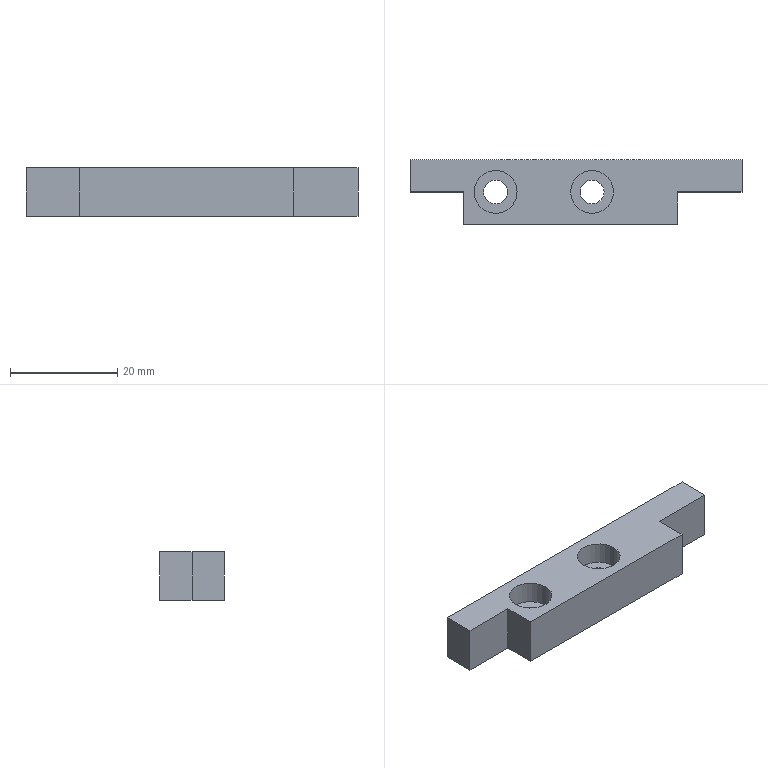Part | STEP file | BU-B02 | 1 solid | 20 faces | box 62 x 12 x 9 mm | volume 4933 mm3 | plane 12 | cylinder 8 | commonest cylinder face diameters 4.5 x4 8 x4
STEP:
#1=CARTESIAN_POINT('',(0.,0.,0.));
#2=DIRECTION('',(0.,0.,1.));
#3=DIRECTION('',(1.,0.,0.));
#4=AXIS2_PLACEMENT_3D('',#1,#2,#3);
#5=CARTESIAN_POINT('',(80.562,56.025,4.8));
#6=VERTEX_POINT('',#5);
#7=CARTESIAN_POINT('',(80.562,56.025,9.));
#8=VERTEX_POINT('',#7);
#9=CARTESIAN_POINT('',(80.562,56.025,9.));
#10=DIRECTION('',(0.,0.,1.));
#11=VECTOR('',#10,1.);
#12=LINE('',#9,#11);
#13=CARTESIAN_POINT('',(76.562,56.025,9.));
#14=DIRECTION('',(0.,0.,1.));
#15=DIRECTION('',(1.,0.,0.));
#16=AXIS2_PLACEMENT_3D('',#13,#14,#15);
#17=CYLINDRICAL_SURFACE('',#16,4.);
#18=CARTESIAN_POINT('',(6.283,0.));
#19=DIRECTION('',(0.,1.));
#20=VECTOR('',#19,1.);
#21=LINE('',#18,#20);
#22=(GEOMETRIC_REPRESENTATION_CONTEXT(2)PARAMETRIC_REPRESENTATION_CONTEXT()REPRESENTATION_CONTEXT('',''));
#23=DEFINITIONAL_REPRESENTATION('',(#21),#22);
#24=PCURVE('',#17,#23);
#25=CARTESIAN_POINT('',(76.562,56.025,9.));
#26=DIRECTION('',(0.,0.,1.));
#27=DIRECTION('',(1.,0.,0.));
#28=AXIS2_PLACEMENT_3D('',#25,#26,#27);
#29=CYLINDRICAL_SURFACE('',#28,4.);
#30=CARTESIAN_POINT('',(0.,0.));
#31=DIRECTION('',(0.,1.));
#32=VECTOR('',#31,1.);
#33=LINE('',#30,#32);
#34=(GEOMETRIC_REPRESENTATION_CONTEXT(2)PARAMETRIC_REPRESENTATION_CONTEXT()REPRESENTATION_CONTEXT('',''));
#35=DEFINITIONAL_REPRESENTATION('',(#33),#34);
#36=PCURVE('',#29,#35);
#37=SURFACE_CURVE('',#12,(#24,#36),.PCURVE_S1.);
#38=EDGE_CURVE('',#6,#8,#37,.T.);
#39=ORIENTED_EDGE('',*,*,#38,.T.);
#40=CARTESIAN_POINT('',(72.562,56.025,9.));
#41=VERTEX_POINT('',#40);
#42=CARTESIAN_POINT('',(76.562,56.025,9.));
#43=DIRECTION('',(0.,0.,1.));
#44=DIRECTION('',(1.,0.,0.));
#45=AXIS2_PLACEMENT_3D('',#42,#43,#44);
#46=CIRCLE('',#45,4.);
#47=CARTESIAN_POINT('',(0.,0.));
#48=DIRECTION('',(1.,0.));
#49=VECTOR('',#48,1.);
#50=LINE('',#47,#49);
#51=(GEOMETRIC_REPRESENTATION_CONTEXT(2)PARAMETRIC_REPRESENTATION_CONTEXT()REPRESENTATION_CONTEXT('',''));
#52=DEFINITIONAL_REPRESENTATION('',(#50),#51);
#53=PCURVE('',#17,#52);
#54=CARTESIAN_POINT('',(60.562,62.025,9.));
#55=DIRECTION('',(0.,0.,-1.));
#56=DIRECTION('',(-1.,0.,0.));
#57=AXIS2_PLACEMENT_3D('',#54,#55,#56);
#58=PLANE('',#57);
#59=CARTESIAN_POINT('',(-20.,-6.));
#60=CARTESIAN_POINT('',(-20.,0.9282));
#61=CARTESIAN_POINT('',(-14.,-2.536));
#62=CARTESIAN_POINT('',(-8.,-6.));
#63=CARTESIAN_POINT('',(-14.,-9.464));
#64=CARTESIAN_POINT('',(-20.,-12.928));
#65=CARTESIAN_POINT('',(-20.,-6.));
#66=(BOUNDED_CURVE()B_SPLINE_CURVE(2,(#59,#60,#61,#62,#63,#64,#65),.UNSPECIFIED.,.T.,.F.)B_SPLINE_CURVE_WITH_KNOTS((1,2,2,2,2,1),(-2.094,0.,2.094,4.189,6.283,8.378),.UNSPECIFIED.)CURVE()GEOMETRIC_REPRESENTATION_ITEM()RATIONAL_B_SPLINE_CURVE((1.,0.5,1.,0.5,1.,0.5,1.))REPRESENTATION_ITEM(''));
#67=(GEOMETRIC_REPRESENTATION_CONTEXT(2)PARAMETRIC_REPRESENTATION_CONTEXT()REPRESENTATION_CONTEXT('',''));
#68=DEFINITIONAL_REPRESENTATION('',(#66),#67);
#69=PCURVE('',#58,#68);
#70=SURFACE_CURVE('',#46,(#53,#69),.PCURVE_S1.);
#71=EDGE_CURVE('',#41,#8,#70,.T.);
#72=ORIENTED_EDGE('',*,*,#71,.F.);
#73=CARTESIAN_POINT('',(72.562,56.025,4.8));
#74=VERTEX_POINT('',#73);
#75=CARTESIAN_POINT('',(72.562,56.025,9.));
#76=DIRECTION('',(0.,0.,1.));
#77=VECTOR('',#76,1.);
#78=LINE('',#75,#77);
#79=CARTESIAN_POINT('',(3.142,0.));
#80=DIRECTION('',(0.,1.));
#81=VECTOR('',#80,1.);
#82=LINE('',#79,#81);
#83=(GEOMETRIC_REPRESENTATION_CONTEXT(2)PARAMETRIC_REPRESENTATION_CONTEXT()REPRESENTATION_CONTEXT('',''));
#84=DEFINITIONAL_REPRESENTATION('',(#82),#83);
#85=PCURVE('',#17,#84);
#86=CARTESIAN_POINT('',(3.142,0.));
#87=DIRECTION('',(0.,1.));
#88=VECTOR('',#87,1.);
#89=LINE('',#86,#88);
#90=(GEOMETRIC_REPRESENTATION_CONTEXT(2)PARAMETRIC_REPRESENTATION_CONTEXT()REPRESENTATION_CONTEXT('',''));
#91=DEFINITIONAL_REPRESENTATION('',(#89),#90);
#92=PCURVE('',#29,#91);
#93=SURFACE_CURVE('',#78,(#85,#92),.PCURVE_S1.);
#94=EDGE_CURVE('',#74,#41,#93,.T.);
#95=ORIENTED_EDGE('',*,*,#94,.F.);
#96=CARTESIAN_POINT('',(76.562,56.025,4.8));
#97=DIRECTION('',(0.,0.,1.));
#98=DIRECTION('',(1.,0.,0.));
#99=AXIS2_PLACEMENT_3D('',#96,#97,#98);
#100=CIRCLE('',#99,4.);
#101=CARTESIAN_POINT('',(0.,-4.2));
#102=DIRECTION('',(1.,0.));
#103=VECTOR('',#102,1.);
#104=LINE('',#101,#103);
#105=(GEOMETRIC_REPRESENTATION_CONTEXT(2)PARAMETRIC_REPRESENTATION_CONTEXT()REPRESENTATION_CONTEXT('',''));
#106=DEFINITIONAL_REPRESENTATION('',(#104),#105);
#107=PCURVE('',#17,#106);
#108=CARTESIAN_POINT('',(78.812,56.025,4.8));
#109=DIRECTION('',(0.,0.,-1.));
#110=DIRECTION('',(-1.,0.,0.));
#111=AXIS2_PLACEMENT_3D('',#108,#109,#110);
#112=PLANE('',#111);
#113=CARTESIAN_POINT('',(-1.75,0.));
#114=CARTESIAN_POINT('',(-1.75,6.928));
#115=CARTESIAN_POINT('',(4.25,3.464));
#116=CARTESIAN_POINT('',(10.25,0.));
#117=CARTESIAN_POINT('',(4.25,-3.464));
#118=CARTESIAN_POINT('',(-1.75,-6.928));
#119=CARTESIAN_POINT('',(-1.75,0.));
#120=(BOUNDED_CURVE()B_SPLINE_CURVE(2,(#113,#114,#115,#116,#117,#118,#119),.UNSPECIFIED.,.T.,.F.)B_SPLINE_CURVE_WITH_KNOTS((1,2,2,2,2,1),(-2.094,0.,2.094,4.189,6.283,8.378),.UNSPECIFIED.)CURVE()GEOMETRIC_REPRESENTATION_ITEM()RATIONAL_B_SPLINE_CURVE((1.,0.5,1.,0.5,1.,0.5,1.))REPRESENTATION_ITEM(''));
#121=(GEOMETRIC_REPRESENTATION_CONTEXT(2)PARAMETRIC_REPRESENTATION_CONTEXT()REPRESENTATION_CONTEXT('',''));
#122=DEFINITIONAL_REPRESENTATION('',(#120),#121);
#123=PCURVE('',#112,#122);
#124=SURFACE_CURVE('',#100,(#107,#123),.PCURVE_S1.);
#125=EDGE_CURVE('',#74,#6,#124,.T.);
#126=ORIENTED_EDGE('',*,*,#125,.T.);
#127=EDGE_LOOP('',(#39,#72,#95,#126));
#128=FACE_BOUND('',#127,.F.);
#129=ADVANCED_FACE('',(#128),#17,.F.);
#130=CARTESIAN_POINT('',(78.812,56.025,0.));
#131=VERTEX_POINT('',#130);
#132=CARTESIAN_POINT('',(78.812,56.025,4.8));
#133=VERTEX_POINT('',#132);
#134=CARTESIAN_POINT('',(78.812,56.025,9.));
#135=DIRECTION('',(0.,0.,1.));
#136=VECTOR('',#135,1.);
#137=LINE('',#134,#136);
#138=CARTESIAN_POINT('',(76.562,56.025,9.));
#139=DIRECTION('',(0.,0.,1.));
#140=DIRECTION('',(1.,0.,0.));
#141=AXIS2_PLACEMENT_3D('',#138,#139,#140);
#142=CYLINDRICAL_SURFACE('',#141,2.25);
#143=CARTESIAN_POINT('',(6.283,0.));
#144=DIRECTION('',(0.,1.));
#145=VECTOR('',#144,1.);
#146=LINE('',#143,#145);
#147=(GEOMETRIC_REPRESENTATION_CONTEXT(2)PARAMETRIC_REPRESENTATION_CONTEXT()REPRESENTATION_CONTEXT('',''));
#148=DEFINITIONAL_REPRESENTATION('',(#146),#147);
#149=PCURVE('',#142,#148);
#150=CARTESIAN_POINT('',(76.562,56.025,9.));
#151=DIRECTION('',(0.,0.,1.));
#152=DIRECTION('',(1.,0.,0.));
#153=AXIS2_PLACEMENT_3D('',#150,#151,#152);
#154=CYLINDRICAL_SURFACE('',#153,2.25);
#155=CARTESIAN_POINT('',(0.,0.));
#156=DIRECTION('',(0.,1.));
#157=VECTOR('',#156,1.);
#158=LINE('',#155,#157);
#159=(GEOMETRIC_REPRESENTATION_CONTEXT(2)PARAMETRIC_REPRESENTATION_CONTEXT()REPRESENTATION_CONTEXT('',''));
#160=DEFINITIONAL_REPRESENTATION('',(#158),#159);
#161=PCURVE('',#154,#160);
#162=SURFACE_CURVE('',#137,(#149,#161),.PCURVE_S1.);
#163=EDGE_CURVE('',#131,#133,#162,.T.);
#164=ORIENTED_EDGE('',*,*,#163,.T.);
#165=CARTESIAN_POINT('',(74.312,56.025,4.8));
#166=VERTEX_POINT('',#165);
#167=CARTESIAN_POINT('',(76.562,56.025,4.8));
#168=DIRECTION('',(0.,0.,1.));
#169=DIRECTION('',(1.,0.,0.));
#170=AXIS2_PLACEMENT_3D('',#167,#168,#169);
#171=CIRCLE('',#170,2.25);
#172=CARTESIAN_POINT('',(0.,-4.2));
#173=DIRECTION('',(1.,0.));
#174=VECTOR('',#173,1.);
#175=LINE('',#172,#174);
#176=(GEOMETRIC_REPRESENTATION_CONTEXT(2)PARAMETRIC_REPRESENTATION_CONTEXT()REPRESENTATION_CONTEXT('',''));
#177=DEFINITIONAL_REPRESENTATION('',(#175),#176);
#178=PCURVE('',#142,#177);
#179=CARTESIAN_POINT('',(0.,0.));
#180=CARTESIAN_POINT('',(0.,3.897));
#181=CARTESIAN_POINT('',(3.375,1.949));
#182=CARTESIAN_POINT('',(6.75,0.));
#183=CARTESIAN_POINT('',(3.375,-1.949));
#184=CARTESIAN_POINT('',(0.,-3.897));
#185=CARTESIAN_POINT('',(0.,0.));
#186=(BOUNDED_CURVE()B_SPLINE_CURVE(2,(#179,#180,#181,#182,#183,#184,#185),.UNSPECIFIED.,.T.,.F.)B_SPLINE_CURVE_WITH_KNOTS((1,2,2,2,2,1),(-2.094,0.,2.094,4.189,6.283,8.378),.UNSPECIFIED.)CURVE()GEOMETRIC_REPRESENTATION_ITEM()RATIONAL_B_SPLINE_CURVE((1.,0.5,1.,0.5,1.,0.5,1.))REPRESENTATION_ITEM(''));
#187=(GEOMETRIC_REPRESENTATION_CONTEXT(2)PARAMETRIC_REPRESENTATION_CONTEXT()REPRESENTATION_CONTEXT('',''));
#188=DEFINITIONAL_REPRESENTATION('',(#186),#187);
#189=PCURVE('',#112,#188);
#190=SURFACE_CURVE('',#171,(#178,#189),.PCURVE_S1.);
#191=EDGE_CURVE('',#166,#133,#190,.T.);
#192=ORIENTED_EDGE('',*,*,#191,.F.);
#193=CARTESIAN_POINT('',(74.312,56.025,0.));
#194=VERTEX_POINT('',#193);
#195=CARTESIAN_POINT('',(74.312,56.025,9.));
#196=DIRECTION('',(0.,0.,1.));
#197=VECTOR('',#196,1.);
#198=LINE('',#195,#197);
#199=CARTESIAN_POINT('',(3.142,0.));
#200=DIRECTION('',(0.,1.));
#201=VECTOR('',#200,1.);
#202=LINE('',#199,#201);
#203=(GEOMETRIC_REPRESENTATION_CONTEXT(2)PARAMETRIC_REPRESENTATION_CONTEXT()REPRESENTATION_CONTEXT('',''));
#204=DEFINITIONAL_REPRESENTATION('',(#202),#203);
#205=PCURVE('',#142,#204);
#206=CARTESIAN_POINT('',(3.142,0.));
#207=DIRECTION('',(0.,1.));
#208=VECTOR('',#207,1.);
#209=LINE('',#206,#208);
#210=(GEOMETRIC_REPRESENTATION_CONTEXT(2)PARAMETRIC_REPRESENTATION_CONTEXT()REPRESENTATION_CONTEXT('',''));
#211=DEFINITIONAL_REPRESENTATION('',(#209),#210);
#212=PCURVE('',#154,#211);
#213=SURFACE_CURVE('',#198,(#205,#212),.PCURVE_S1.);
#214=EDGE_CURVE('',#194,#166,#213,.T.);
#215=ORIENTED_EDGE('',*,*,#214,.F.);
#216=CARTESIAN_POINT('',(76.562,56.025,0.));
#217=DIRECTION('',(0.,0.,-1.));
#218=DIRECTION('',(-1.,0.,0.));
#219=AXIS2_PLACEMENT_3D('',#216,#217,#218);
#220=CIRCLE('',#219,2.25);
#221=CARTESIAN_POINT('',(9.425,-9.));
#222=DIRECTION('',(-1.,0.));
#223=VECTOR('',#222,1.);
#224=LINE('',#221,#223);
#225=(GEOMETRIC_REPRESENTATION_CONTEXT(2)PARAMETRIC_REPRESENTATION_CONTEXT()REPRESENTATION_CONTEXT('',''));
#226=DEFINITIONAL_REPRESENTATION('',(#224),#225);
#227=PCURVE('',#142,#226);
#228=CARTESIAN_POINT('',(60.562,62.025,0.));
#229=DIRECTION('',(0.,0.,-1.));
#230=DIRECTION('',(-1.,0.,0.));
#231=AXIS2_PLACEMENT_3D('',#228,#229,#230);
#232=PLANE('',#231);
#233=CARTESIAN_POINT('',(-16.,-6.));
#234=DIRECTION('',(1.,0.));
#235=AXIS2_PLACEMENT_2D('',#233,#234);
#236=CIRCLE('',#235,2.25);
#237=(GEOMETRIC_REPRESENTATION_CONTEXT(2)PARAMETRIC_REPRESENTATION_CONTEXT()REPRESENTATION_CONTEXT('',''));
#238=DEFINITIONAL_REPRESENTATION('',(#236),#237);
#239=PCURVE('',#232,#238);
#240=SURFACE_CURVE('',#220,(#227,#239),.PCURVE_S1.);
#241=EDGE_CURVE('',#131,#194,#240,.T.);
#242=ORIENTED_EDGE('',*,*,#241,.F.);
#243=EDGE_LOOP('',(#164,#192,#215,#242));
#244=FACE_BOUND('',#243,.F.);
#245=ADVANCED_FACE('',(#244),#142,.F.);
#246=CARTESIAN_POINT('',(98.562,56.025,4.8));
#247=VERTEX_POINT('',#246);
#248=CARTESIAN_POINT('',(98.562,56.025,9.));
#249=VERTEX_POINT('',#248);
#250=CARTESIAN_POINT('',(98.562,56.025,9.));
#251=DIRECTION('',(0.,0.,1.));
#252=VECTOR('',#251,1.);
#253=LINE('',#250,#252);
#254=CARTESIAN_POINT('',(94.562,56.025,9.));
#255=DIRECTION('',(0.,0.,1.));
#256=DIRECTION('',(1.,0.,0.));
#257=AXIS2_PLACEMENT_3D('',#254,#255,#256);
#258=CYLINDRICAL_SURFACE('',#257,4.);
#259=CARTESIAN_POINT('',(6.283,0.));
#260=DIRECTION('',(0.,1.));
#261=VECTOR('',#260,1.);
#262=LINE('',#259,#261);
#263=(GEOMETRIC_REPRESENTATION_CONTEXT(2)PARAMETRIC_REPRESENTATION_CONTEXT()REPRESENTATION_CONTEXT('',''));
#264=DEFINITIONAL_REPRESENTATION('',(#262),#263);
#265=PCURVE('',#258,#264);
#266=CARTESIAN_POINT('',(94.562,56.025,9.));
#267=DIRECTION('',(0.,0.,1.));
#268=DIRECTION('',(1.,0.,0.));
#269=AXIS2_PLACEMENT_3D('',#266,#267,#268);
#270=CYLINDRICAL_SURFACE('',#269,4.);
#271=CARTESIAN_POINT('',(0.,0.));
#272=DIRECTION('',(0.,1.));
#273=VECTOR('',#272,1.);
#274=LINE('',#271,#273);
#275=(GEOMETRIC_REPRESENTATION_CONTEXT(2)PARAMETRIC_REPRESENTATION_CONTEXT()REPRESENTATION_CONTEXT('',''));
#276=DEFINITIONAL_REPRESENTATION('',(#274),#275);
#277=PCURVE('',#270,#276);
#278=SURFACE_CURVE('',#253,(#265,#277),.PCURVE_S1.);
#279=EDGE_CURVE('',#247,#249,#278,.T.);
#280=ORIENTED_EDGE('',*,*,#279,.T.);
#281=CARTESIAN_POINT('',(90.562,56.025,9.));
#282=VERTEX_POINT('',#281);
#283=CARTESIAN_POINT('',(94.562,56.025,9.));
#284=DIRECTION('',(0.,0.,1.));
#285=DIRECTION('',(1.,0.,0.));
#286=AXIS2_PLACEMENT_3D('',#283,#284,#285);
#287=CIRCLE('',#286,4.);
#288=CARTESIAN_POINT('',(0.,0.));
#289=DIRECTION('',(1.,0.));
#290=VECTOR('',#289,1.);
#291=LINE('',#288,#290);
#292=(GEOMETRIC_REPRESENTATION_CONTEXT(2)PARAMETRIC_REPRESENTATION_CONTEXT()REPRESENTATION_CONTEXT('',''));
#293=DEFINITIONAL_REPRESENTATION('',(#291),#292);
#294=PCURVE('',#258,#293);
#295=CARTESIAN_POINT('',(-38.,-6.));
#296=CARTESIAN_POINT('',(-38.,0.9282));
#297=CARTESIAN_POINT('',(-32.,-2.536));
#298=CARTESIAN_POINT('',(-26.,-6.));
#299=CARTESIAN_POINT('',(-32.,-9.464));
#300=CARTESIAN_POINT('',(-38.,-12.928));
#301=CARTESIAN_POINT('',(-38.,-6.));
#302=(BOUNDED_CURVE()B_SPLINE_CURVE(2,(#295,#296,#297,#298,#299,#300,#301),.UNSPECIFIED.,.T.,.F.)B_SPLINE_CURVE_WITH_KNOTS((1,2,2,2,2,1),(-2.094,0.,2.094,4.189,6.283,8.378),.UNSPECIFIED.)CURVE()GEOMETRIC_REPRESENTATION_ITEM()RATIONAL_B_SPLINE_CURVE((1.,0.5,1.,0.5,1.,0.5,1.))REPRESENTATION_ITEM(''));
#303=(GEOMETRIC_REPRESENTATION_CONTEXT(2)PARAMETRIC_REPRESENTATION_CONTEXT()REPRESENTATION_CONTEXT('',''));
#304=DEFINITIONAL_REPRESENTATION('',(#302),#303);
#305=PCURVE('',#58,#304);
#306=SURFACE_CURVE('',#287,(#294,#305),.PCURVE_S1.);
#307=EDGE_CURVE('',#282,#249,#306,.T.);
#308=ORIENTED_EDGE('',*,*,#307,.F.);
#309=CARTESIAN_POINT('',(90.562,56.025,4.8));
#310=VERTEX_POINT('',#309);
#311=CARTESIAN_POINT('',(90.562,56.025,9.));
#312=DIRECTION('',(0.,0.,1.));
#313=VECTOR('',#312,1.);
#314=LINE('',#311,#313);
#315=CARTESIAN_POINT('',(3.142,0.));
#316=DIRECTION('',(0.,1.));
#317=VECTOR('',#316,1.);
#318=LINE('',#315,#317);
#319=(GEOMETRIC_REPRESENTATION_CONTEXT(2)PARAMETRIC_REPRESENTATION_CONTEXT()REPRESENTATION_CONTEXT('',''));
#320=DEFINITIONAL_REPRESENTATION('',(#318),#319);
#321=PCURVE('',#258,#320);
#322=CARTESIAN_POINT('',(3.142,0.));
#323=DIRECTION('',(0.,1.));
#324=VECTOR('',#323,1.);
#325=LINE('',#322,#324);
#326=(GEOMETRIC_REPRESENTATION_CONTEXT(2)PARAMETRIC_REPRESENTATION_CONTEXT()REPRESENTATION_CONTEXT('',''));
#327=DEFINITIONAL_REPRESENTATION('',(#325),#326);
#328=PCURVE('',#270,#327);
#329=SURFACE_CURVE('',#314,(#321,#328),.PCURVE_S1.);
#330=EDGE_CURVE('',#310,#282,#329,.T.);
#331=ORIENTED_EDGE('',*,*,#330,.F.);
#332=CARTESIAN_POINT('',(94.562,56.025,4.8));
#333=DIRECTION('',(0.,0.,1.));
#334=DIRECTION('',(1.,0.,0.));
#335=AXIS2_PLACEMENT_3D('',#332,#333,#334);
#336=CIRCLE('',#335,4.);
#337=CARTESIAN_POINT('',(0.,-4.2));
#338=DIRECTION('',(1.,0.));
#339=VECTOR('',#338,1.);
#340=LINE('',#337,#339);
#341=(GEOMETRIC_REPRESENTATION_CONTEXT(2)PARAMETRIC_REPRESENTATION_CONTEXT()REPRESENTATION_CONTEXT('',''));
#342=DEFINITIONAL_REPRESENTATION('',(#340),#341);
#343=PCURVE('',#258,#342);
#344=CARTESIAN_POINT('',(96.812,56.025,4.8));
#345=DIRECTION('',(0.,0.,-1.));
#346=DIRECTION('',(-1.,0.,0.));
#347=AXIS2_PLACEMENT_3D('',#344,#345,#346);
#348=PLANE('',#347);
#349=CARTESIAN_POINT('',(-1.75,0.));
#350=CARTESIAN_POINT('',(-1.75,6.928));
#351=CARTESIAN_POINT('',(4.25,3.464));
#352=CARTESIAN_POINT('',(10.25,0.));
#353=CARTESIAN_POINT('',(4.25,-3.464));
#354=CARTESIAN_POINT('',(-1.75,-6.928));
#355=CARTESIAN_POINT('',(-1.75,0.));
#356=(BOUNDED_CURVE()B_SPLINE_CURVE(2,(#349,#350,#351,#352,#353,#354,#355),.UNSPECIFIED.,.T.,.F.)B_SPLINE_CURVE_WITH_KNOTS((1,2,2,2,2,1),(-2.094,0.,2.094,4.189,6.283,8.378),.UNSPECIFIED.)CURVE()GEOMETRIC_REPRESENTATION_ITEM()RATIONAL_B_SPLINE_CURVE((1.,0.5,1.,0.5,1.,0.5,1.))REPRESENTATION_ITEM(''));
#357=(GEOMETRIC_REPRESENTATION_CONTEXT(2)PARAMETRIC_REPRESENTATION_CONTEXT()REPRESENTATION_CONTEXT('',''));
#358=DEFINITIONAL_REPRESENTATION('',(#356),#357);
#359=PCURVE('',#348,#358);
#360=SURFACE_CURVE('',#336,(#343,#359),.PCURVE_S1.);
#361=EDGE_CURVE('',#310,#247,#360,.T.);
#362=ORIENTED_EDGE('',*,*,#361,.T.);
#363=EDGE_LOOP('',(#280,#308,#331,#362));
#364=FACE_BOUND('',#363,.F.);
#365=ADVANCED_FACE('',(#364),#258,.F.);
#366=CARTESIAN_POINT('',(96.812,56.025,0.));
#367=VERTEX_POINT('',#366);
#368=CARTESIAN_POINT('',(96.812,56.025,4.8));
#369=VERTEX_POINT('',#368);
#370=CARTESIAN_POINT('',(96.812,56.025,9.));
#371=DIRECTION('',(0.,0.,1.));
#372=VECTOR('',#371,1.);
#373=LINE('',#370,#372);
#374=CARTESIAN_POINT('',(94.562,56.025,9.));
#375=DIRECTION('',(0.,0.,1.));
#376=DIRECTION('',(1.,0.,0.));
#377=AXIS2_PLACEMENT_3D('',#374,#375,#376);
#378=CYLINDRICAL_SURFACE('',#377,2.25);
#379=CARTESIAN_POINT('',(6.283,0.));
#380=DIRECTION('',(0.,1.));
#381=VECTOR('',#380,1.);
#382=LINE('',#379,#381);
#383=(GEOMETRIC_REPRESENTATION_CONTEXT(2)PARAMETRIC_REPRESENTATION_CONTEXT()REPRESENTATION_CONTEXT('',''));
#384=DEFINITIONAL_REPRESENTATION('',(#382),#383);
#385=PCURVE('',#378,#384);
#386=CARTESIAN_POINT('',(94.562,56.025,9.));
#387=DIRECTION('',(0.,0.,1.));
#388=DIRECTION('',(1.,0.,0.));
#389=AXIS2_PLACEMENT_3D('',#386,#387,#388);
#390=CYLINDRICAL_SURFACE('',#389,2.25);
#391=CARTESIAN_POINT('',(0.,0.));
#392=DIRECTION('',(0.,1.));
#393=VECTOR('',#392,1.);
#394=LINE('',#391,#393);
#395=(GEOMETRIC_REPRESENTATION_CONTEXT(2)PARAMETRIC_REPRESENTATION_CONTEXT()REPRESENTATION_CONTEXT('',''));
#396=DEFINITIONAL_REPRESENTATION('',(#394),#395);
#397=PCURVE('',#390,#396);
#398=SURFACE_CURVE('',#373,(#385,#397),.PCURVE_S1.);
#399=EDGE_CURVE('',#367,#369,#398,.T.);
#400=ORIENTED_EDGE('',*,*,#399,.T.);
#401=CARTESIAN_POINT('',(92.312,56.025,4.8));
#402=VERTEX_POINT('',#401);
#403=CARTESIAN_POINT('',(94.562,56.025,4.8));
#404=DIRECTION('',(0.,0.,1.));
#405=DIRECTION('',(1.,0.,0.));
#406=AXIS2_PLACEMENT_3D('',#403,#404,#405);
#407=CIRCLE('',#406,2.25);
#408=CARTESIAN_POINT('',(0.,-4.2));
#409=DIRECTION('',(1.,0.));
#410=VECTOR('',#409,1.);
#411=LINE('',#408,#410);
#412=(GEOMETRIC_REPRESENTATION_CONTEXT(2)PARAMETRIC_REPRESENTATION_CONTEXT()REPRESENTATION_CONTEXT('',''));
#413=DEFINITIONAL_REPRESENTATION('',(#411),#412);
#414=PCURVE('',#378,#413);
#415=CARTESIAN_POINT('',(0.,0.));
#416=CARTESIAN_POINT('',(0.,3.897));
#417=CARTESIAN_POINT('',(3.375,1.949));
#418=CARTESIAN_POINT('',(6.75,0.));
#419=CARTESIAN_POINT('',(3.375,-1.949));
#420=CARTESIAN_POINT('',(0.,-3.897));
#421=CARTESIAN_POINT('',(0.,0.));
#422=(BOUNDED_CURVE()B_SPLINE_CURVE(2,(#415,#416,#417,#418,#419,#420,#421),.UNSPECIFIED.,.T.,.F.)B_SPLINE_CURVE_WITH_KNOTS((1,2,2,2,2,1),(-2.094,0.,2.094,4.189,6.283,8.378),.UNSPECIFIED.)CURVE()GEOMETRIC_REPRESENTATION_ITEM()RATIONAL_B_SPLINE_CURVE((1.,0.5,1.,0.5,1.,0.5,1.))REPRESENTATION_ITEM(''));
#423=(GEOMETRIC_REPRESENTATION_CONTEXT(2)PARAMETRIC_REPRESENTATION_CONTEXT()REPRESENTATION_CONTEXT('',''));
#424=DEFINITIONAL_REPRESENTATION('',(#422),#423);
#425=PCURVE('',#348,#424);
#426=SURFACE_CURVE('',#407,(#414,#425),.PCURVE_S1.);
#427=EDGE_CURVE('',#402,#369,#426,.T.);
#428=ORIENTED_EDGE('',*,*,#427,.F.);
#429=CARTESIAN_POINT('',(92.312,56.025,0.));
#430=VERTEX_POINT('',#429);
#431=CARTESIAN_POINT('',(92.312,56.025,9.));
#432=DIRECTION('',(0.,0.,1.));
#433=VECTOR('',#432,1.);
#434=LINE('',#431,#433);
#435=CARTESIAN_POINT('',(3.142,0.));
#436=DIRECTION('',(0.,1.));
#437=VECTOR('',#436,1.);
#438=LINE('',#435,#437);
#439=(GEOMETRIC_REPRESENTATION_CONTEXT(2)PARAMETRIC_REPRESENTATION_CONTEXT()REPRESENTATION_CONTEXT('',''));
#440=DEFINITIONAL_REPRESENTATION('',(#438),#439);
#441=PCURVE('',#378,#440);
#442=CARTESIAN_POINT('',(3.142,0.));
#443=DIRECTION('',(0.,1.));
#444=VECTOR('',#443,1.);
#445=LINE('',#442,#444);
#446=(GEOMETRIC_REPRESENTATION_CONTEXT(2)PARAMETRIC_REPRESENTATION_CONTEXT()REPRESENTATION_CONTEXT('',''));
#447=DEFINITIONAL_REPRESENTATION('',(#445),#446);
#448=PCURVE('',#390,#447);
#449=SURFACE_CURVE('',#434,(#441,#448),.PCURVE_S1.);
#450=EDGE_CURVE('',#430,#402,#449,.T.);
#451=ORIENTED_EDGE('',*,*,#450,.F.);
#452=CARTESIAN_POINT('',(94.562,56.025,0.));
#453=DIRECTION('',(0.,0.,-1.));
#454=DIRECTION('',(-1.,0.,0.));
#455=AXIS2_PLACEMENT_3D('',#452,#453,#454);
#456=CIRCLE('',#455,2.25);
#457=CARTESIAN_POINT('',(9.425,-9.));
#458=DIRECTION('',(-1.,0.));
#459=VECTOR('',#458,1.);
#460=LINE('',#457,#459);
#461=(GEOMETRIC_REPRESENTATION_CONTEXT(2)PARAMETRIC_REPRESENTATION_CONTEXT()REPRESENTATION_CONTEXT('',''));
#462=DEFINITIONAL_REPRESENTATION('',(#460),#461);
#463=PCURVE('',#378,#462);
#464=CARTESIAN_POINT('',(-34.,-6.));
#465=DIRECTION('',(1.,0.));
#466=AXIS2_PLACEMENT_2D('',#464,#465);
#467=CIRCLE('',#466,2.25);
#468=(GEOMETRIC_REPRESENTATION_CONTEXT(2)PARAMETRIC_REPRESENTATION_CONTEXT()REPRESENTATION_CONTEXT('',''));
#469=DEFINITIONAL_REPRESENTATION('',(#467),#468);
#470=PCURVE('',#232,#469);
#471=SURFACE_CURVE('',#456,(#463,#470),.PCURVE_S1.);
#472=EDGE_CURVE('',#367,#430,#471,.T.);
#473=ORIENTED_EDGE('',*,*,#472,.F.);
#474=EDGE_LOOP('',(#400,#428,#451,#473));
#475=FACE_BOUND('',#474,.F.);
#476=ADVANCED_FACE('',(#475),#378,.F.);
#477=CARTESIAN_POINT('',(60.562,62.025,0.));
#478=VERTEX_POINT('',#477);
#479=CARTESIAN_POINT('',(60.562,56.025,0.));
#480=VERTEX_POINT('',#479);
#481=CARTESIAN_POINT('',(60.562,56.025,0.));
#482=DIRECTION('',(0.,-1.,0.));
#483=VECTOR('',#482,1.);
#484=LINE('',#481,#483);
#485=CARTESIAN_POINT('',(60.562,56.025,9.));
#486=DIRECTION('',(1.,0.,0.));
#487=DIRECTION('',(0.,0.,-1.));
#488=AXIS2_PLACEMENT_3D('',#485,#486,#487);
#489=PLANE('',#488);
#490=CARTESIAN_POINT('',(9.,0.));
#491=DIRECTION('',(0.,-1.));
#492=VECTOR('',#491,1.);
#493=LINE('',#490,#492);
#494=(GEOMETRIC_REPRESENTATION_CONTEXT(2)PARAMETRIC_REPRESENTATION_CONTEXT()REPRESENTATION_CONTEXT('',''));
#495=DEFINITIONAL_REPRESENTATION('',(#493),#494);
#496=PCURVE('',#489,#495);
#497=CARTESIAN_POINT('',(0.,-6.));
#498=DIRECTION('',(0.,-1.));
#499=VECTOR('',#498,1.);
#500=LINE('',#497,#499);
#501=(GEOMETRIC_REPRESENTATION_CONTEXT(2)PARAMETRIC_REPRESENTATION_CONTEXT()REPRESENTATION_CONTEXT('',''));
#502=DEFINITIONAL_REPRESENTATION('',(#500),#501);
#503=PCURVE('',#232,#502);
#504=SURFACE_CURVE('',#484,(#496,#503),.PCURVE_S1.);
#505=EDGE_CURVE('',#478,#480,#504,.T.);
#506=ORIENTED_EDGE('',*,*,#505,.T.);
#507=CARTESIAN_POINT('',(60.562,56.025,9.));
#508=VERTEX_POINT('',#507);
#509=CARTESIAN_POINT('',(60.562,56.025,9.));
#510=DIRECTION('',(0.,0.,-1.));
#511=VECTOR('',#510,1.);
#512=LINE('',#509,#511);
#513=CARTESIAN_POINT('',(0.,0.));
#514=DIRECTION('',(1.,0.));
#515=VECTOR('',#514,1.);
#516=LINE('',#513,#515);
#517=(GEOMETRIC_REPRESENTATION_CONTEXT(2)PARAMETRIC_REPRESENTATION_CONTEXT()REPRESENTATION_CONTEXT('',''));
#518=DEFINITIONAL_REPRESENTATION('',(#516),#517);
#519=PCURVE('',#489,#518);
#520=CARTESIAN_POINT('',(60.562,56.025,9.));
#521=DIRECTION('',(0.,1.,0.));
#522=DIRECTION('',(0.,0.,1.));
#523=AXIS2_PLACEMENT_3D('',#520,#521,#522);
#524=PLANE('',#523);
#525=CARTESIAN_POINT('',(0.,0.));
#526=DIRECTION('',(-1.,0.));
#527=VECTOR('',#526,1.);
#528=LINE('',#525,#527);
#529=(GEOMETRIC_REPRESENTATION_CONTEXT(2)PARAMETRIC_REPRESENTATION_CONTEXT()REPRESENTATION_CONTEXT('',''));
#530=DEFINITIONAL_REPRESENTATION('',(#528),#529);
#531=PCURVE('',#524,#530);
#532=SURFACE_CURVE('',#512,(#519,#531),.PCURVE_S1.);
#533=EDGE_CURVE('',#508,#480,#532,.T.);
#534=ORIENTED_EDGE('',*,*,#533,.F.);
#535=CARTESIAN_POINT('',(60.562,62.025,9.));
#536=VERTEX_POINT('',#535);
#537=CARTESIAN_POINT('',(60.562,56.025,9.));
#538=DIRECTION('',(0.,-1.,0.));
#539=VECTOR('',#538,1.);
#540=LINE('',#537,#539);
#541=CARTESIAN_POINT('',(0.,0.));
#542=DIRECTION('',(0.,-1.));
#543=VECTOR('',#542,1.);
#544=LINE('',#541,#543);
#545=(GEOMETRIC_REPRESENTATION_CONTEXT(2)PARAMETRIC_REPRESENTATION_CONTEXT()REPRESENTATION_CONTEXT('',''));
#546=DEFINITIONAL_REPRESENTATION('',(#544),#545);
#547=PCURVE('',#489,#546);
#548=CARTESIAN_POINT('',(0.,-6.));
#549=DIRECTION('',(0.,-1.));
#550=VECTOR('',#549,1.);
#551=LINE('',#548,#550);
#552=(GEOMETRIC_REPRESENTATION_CONTEXT(2)PARAMETRIC_REPRESENTATION_CONTEXT()REPRESENTATION_CONTEXT('',''));
#553=DEFINITIONAL_REPRESENTATION('',(#551),#552);
#554=PCURVE('',#58,#553);
#555=SURFACE_CURVE('',#540,(#547,#554),.PCURVE_S1.);
#556=EDGE_CURVE('',#536,#508,#555,.T.);
#557=ORIENTED_EDGE('',*,*,#556,.F.);
#558=CARTESIAN_POINT('',(60.562,62.025,9.));
#559=DIRECTION('',(0.,0.,-1.));
#560=VECTOR('',#559,1.);
#561=LINE('',#558,#560);
#562=CARTESIAN_POINT('',(0.,6.));
#563=DIRECTION('',(1.,0.));
#564=VECTOR('',#563,1.);
#565=LINE('',#562,#564);
#566=(GEOMETRIC_REPRESENTATION_CONTEXT(2)PARAMETRIC_REPRESENTATION_CONTEXT()REPRESENTATION_CONTEXT('',''));
#567=DEFINITIONAL_REPRESENTATION('',(#565),#566);
#568=PCURVE('',#489,#567);
#569=CARTESIAN_POINT('',(60.562,62.025,9.));
#570=DIRECTION('',(0.,-1.,0.));
#571=DIRECTION('',(0.,0.,-1.));
#572=AXIS2_PLACEMENT_3D('',#569,#570,#571);
#573=PLANE('',#572);
#574=CARTESIAN_POINT('',(0.,0.));
#575=DIRECTION('',(1.,0.));
#576=VECTOR('',#575,1.);
#577=LINE('',#574,#576);
#578=(GEOMETRIC_REPRESENTATION_CONTEXT(2)PARAMETRIC_REPRESENTATION_CONTEXT()REPRESENTATION_CONTEXT('',''));
#579=DEFINITIONAL_REPRESENTATION('',(#577),#578);
#580=PCURVE('',#573,#579);
#581=SURFACE_CURVE('',#561,(#568,#580),.PCURVE_S1.);
#582=EDGE_CURVE('',#536,#478,#581,.T.);
#583=ORIENTED_EDGE('',*,*,#582,.T.);
#584=EDGE_LOOP('',(#506,#534,#557,#583));
#585=FACE_BOUND('',#584,.T.);
#586=ADVANCED_FACE('',(#585),#489,.F.);
#587=CARTESIAN_POINT('',(70.562,56.025,0.));
#588=VERTEX_POINT('',#587);
#589=CARTESIAN_POINT('',(60.562,56.025,0.));
#590=DIRECTION('',(1.,0.,0.));
#591=VECTOR('',#590,1.);
#592=LINE('',#589,#591);
#593=CARTESIAN_POINT('',(-9.,0.));
#594=DIRECTION('',(0.,1.));
#595=VECTOR('',#594,1.);
#596=LINE('',#593,#595);
#597=(GEOMETRIC_REPRESENTATION_CONTEXT(2)PARAMETRIC_REPRESENTATION_CONTEXT()REPRESENTATION_CONTEXT('',''));
#598=DEFINITIONAL_REPRESENTATION('',(#596),#597);
#599=PCURVE('',#524,#598);
#600=CARTESIAN_POINT('',(0.,-6.));
#601=DIRECTION('',(-1.,0.));
#602=VECTOR('',#601,1.);
#603=LINE('',#600,#602);
#604=(GEOMETRIC_REPRESENTATION_CONTEXT(2)PARAMETRIC_REPRESENTATION_CONTEXT()REPRESENTATION_CONTEXT('',''));
#605=DEFINITIONAL_REPRESENTATION('',(#603),#604);
#606=PCURVE('',#232,#605);
#607=SURFACE_CURVE('',#592,(#599,#606),.PCURVE_S1.);
#608=EDGE_CURVE('',#480,#588,#607,.T.);
#609=ORIENTED_EDGE('',*,*,#608,.T.);
#610=CARTESIAN_POINT('',(70.562,56.025,9.));
#611=VERTEX_POINT('',#610);
#612=CARTESIAN_POINT('',(70.562,56.025,9.));
#613=DIRECTION('',(0.,0.,-1.));
#614=VECTOR('',#613,1.);
#615=LINE('',#612,#614);
#616=CARTESIAN_POINT('',(0.,10.));
#617=DIRECTION('',(-1.,0.));
#618=VECTOR('',#617,1.);
#619=LINE('',#616,#618);
#620=(GEOMETRIC_REPRESENTATION_CONTEXT(2)PARAMETRIC_REPRESENTATION_CONTEXT()REPRESENTATION_CONTEXT('',''));
#621=DEFINITIONAL_REPRESENTATION('',(#619),#620);
#622=PCURVE('',#524,#621);
#623=CARTESIAN_POINT('',(70.562,56.025,9.));
#624=DIRECTION('',(1.,0.,0.));
#625=DIRECTION('',(0.,0.,-1.));
#626=AXIS2_PLACEMENT_3D('',#623,#624,#625);
#627=PLANE('',#626);
#628=CARTESIAN_POINT('',(0.,0.));
#629=DIRECTION('',(1.,0.));
#630=VECTOR('',#629,1.);
#631=LINE('',#628,#630);
#632=(GEOMETRIC_REPRESENTATION_CONTEXT(2)PARAMETRIC_REPRESENTATION_CONTEXT()REPRESENTATION_CONTEXT('',''));
#633=DEFINITIONAL_REPRESENTATION('',(#631),#632);
#634=PCURVE('',#627,#633);
#635=SURFACE_CURVE('',#615,(#622,#634),.PCURVE_S1.);
#636=EDGE_CURVE('',#611,#588,#635,.T.);
#637=ORIENTED_EDGE('',*,*,#636,.F.);
#638=CARTESIAN_POINT('',(60.562,56.025,9.));
#639=DIRECTION('',(1.,0.,0.));
#640=VECTOR('',#639,1.);
#641=LINE('',#638,#640);
#642=CARTESIAN_POINT('',(0.,0.));
#643=DIRECTION('',(0.,1.));
#644=VECTOR('',#643,1.);
#645=LINE('',#642,#644);
#646=(GEOMETRIC_REPRESENTATION_CONTEXT(2)PARAMETRIC_REPRESENTATION_CONTEXT()REPRESENTATION_CONTEXT('',''));
#647=DEFINITIONAL_REPRESENTATION('',(#645),#646);
#648=PCURVE('',#524,#647);
#649=CARTESIAN_POINT('',(0.,-6.));
#650=DIRECTION('',(-1.,0.));
#651=VECTOR('',#650,1.);
#652=LINE('',#649,#651);
#653=(GEOMETRIC_REPRESENTATION_CONTEXT(2)PARAMETRIC_REPRESENTATION_CONTEXT()REPRESENTATION_CONTEXT('',''));
#654=DEFINITIONAL_REPRESENTATION('',(#652),#653);
#655=PCURVE('',#58,#654);
#656=SURFACE_CURVE('',#641,(#648,#655),.PCURVE_S1.);
#657=EDGE_CURVE('',#508,#611,#656,.T.);
#658=ORIENTED_EDGE('',*,*,#657,.F.);
#659=ORIENTED_EDGE('',*,*,#533,.T.);
#660=EDGE_LOOP('',(#609,#637,#658,#659));
#661=FACE_BOUND('',#660,.T.);
#662=ADVANCED_FACE('',(#661),#524,.F.);
#663=CARTESIAN_POINT('',(70.562,50.025,0.));
#664=VERTEX_POINT('',#663);
#665=CARTESIAN_POINT('',(70.562,56.025,0.));
#666=DIRECTION('',(0.,-1.,0.));
#667=VECTOR('',#666,1.);
#668=LINE('',#665,#667);
#669=CARTESIAN_POINT('',(9.,0.));
#670=DIRECTION('',(0.,-1.));
#671=VECTOR('',#670,1.);
#672=LINE('',#669,#671);
#673=(GEOMETRIC_REPRESENTATION_CONTEXT(2)PARAMETRIC_REPRESENTATION_CONTEXT()REPRESENTATION_CONTEXT('',''));
#674=DEFINITIONAL_REPRESENTATION('',(#672),#673);
#675=PCURVE('',#627,#674);
#676=CARTESIAN_POINT('',(-10.,-6.));
#677=DIRECTION('',(0.,-1.));
#678=VECTOR('',#677,1.);
#679=LINE('',#676,#678);
#680=(GEOMETRIC_REPRESENTATION_CONTEXT(2)PARAMETRIC_REPRESENTATION_CONTEXT()REPRESENTATION_CONTEXT('',''));
#681=DEFINITIONAL_REPRESENTATION('',(#679),#680);
#682=PCURVE('',#232,#681);
#683=SURFACE_CURVE('',#668,(#675,#682),.PCURVE_S1.);
#684=EDGE_CURVE('',#588,#664,#683,.T.);
#685=ORIENTED_EDGE('',*,*,#684,.T.);
#686=CARTESIAN_POINT('',(70.562,50.025,9.));
#687=VERTEX_POINT('',#686);
#688=CARTESIAN_POINT('',(70.562,50.025,9.));
#689=DIRECTION('',(0.,0.,-1.));
#690=VECTOR('',#689,1.);
#691=LINE('',#688,#690);
#692=CARTESIAN_POINT('',(0.,-6.));
#693=DIRECTION('',(1.,0.));
#694=VECTOR('',#693,1.);
#695=LINE('',#692,#694);
#696=(GEOMETRIC_REPRESENTATION_CONTEXT(2)PARAMETRIC_REPRESENTATION_CONTEXT()REPRESENTATION_CONTEXT('',''));
#697=DEFINITIONAL_REPRESENTATION('',(#695),#696);
#698=PCURVE('',#627,#697);
#699=CARTESIAN_POINT('',(70.562,50.025,9.));
#700=DIRECTION('',(0.,1.,0.));
#701=DIRECTION('',(-1.,0.,0.));
#702=AXIS2_PLACEMENT_3D('',#699,#700,#701);
#703=PLANE('',#702);
#704=CARTESIAN_POINT('',(0.,0.));
#705=DIRECTION('',(0.,-1.));
#706=VECTOR('',#705,1.);
#707=LINE('',#704,#706);
#708=(GEOMETRIC_REPRESENTATION_CONTEXT(2)PARAMETRIC_REPRESENTATION_CONTEXT()REPRESENTATION_CONTEXT('',''));
#709=DEFINITIONAL_REPRESENTATION('',(#707),#708);
#710=PCURVE('',#703,#709);
#711=SURFACE_CURVE('',#691,(#698,#710),.PCURVE_S1.);
#712=EDGE_CURVE('',#687,#664,#711,.T.);
#713=ORIENTED_EDGE('',*,*,#712,.F.);
#714=CARTESIAN_POINT('',(70.562,56.025,9.));
#715=DIRECTION('',(0.,-1.,0.));
#716=VECTOR('',#715,1.);
#717=LINE('',#714,#716);
#718=CARTESIAN_POINT('',(0.,0.));
#719=DIRECTION('',(0.,-1.));
#720=VECTOR('',#719,1.);
#721=LINE('',#718,#720);
#722=(GEOMETRIC_REPRESENTATION_CONTEXT(2)PARAMETRIC_REPRESENTATION_CONTEXT()REPRESENTATION_CONTEXT('',''));
#723=DEFINITIONAL_REPRESENTATION('',(#721),#722);
#724=PCURVE('',#627,#723);
#725=CARTESIAN_POINT('',(-10.,-6.));
#726=DIRECTION('',(0.,-1.));
#727=VECTOR('',#726,1.);
#728=LINE('',#725,#727);
#729=(GEOMETRIC_REPRESENTATION_CONTEXT(2)PARAMETRIC_REPRESENTATION_CONTEXT()REPRESENTATION_CONTEXT('',''));
#730=DEFINITIONAL_REPRESENTATION('',(#728),#729);
#731=PCURVE('',#58,#730);
#732=SURFACE_CURVE('',#717,(#724,#731),.PCURVE_S1.);
#733=EDGE_CURVE('',#611,#687,#732,.T.);
#734=ORIENTED_EDGE('',*,*,#733,.F.);
#735=ORIENTED_EDGE('',*,*,#636,.T.);
#736=EDGE_LOOP('',(#685,#713,#734,#735));
#737=FACE_BOUND('',#736,.T.);
#738=ADVANCED_FACE('',(#737),#627,.F.);
#739=CARTESIAN_POINT('',(110.562,50.025,0.));
#740=VERTEX_POINT('',#739);
#741=CARTESIAN_POINT('',(70.562,50.025,0.));
#742=DIRECTION('',(1.,0.,0.));
#743=VECTOR('',#742,1.);
#744=LINE('',#741,#743);
#745=CARTESIAN_POINT('',(0.,-9.));
#746=DIRECTION('',(-1.,0.));
#747=VECTOR('',#746,1.);
#748=LINE('',#745,#747);
#749=(GEOMETRIC_REPRESENTATION_CONTEXT(2)PARAMETRIC_REPRESENTATION_CONTEXT()REPRESENTATION_CONTEXT('',''));
#750=DEFINITIONAL_REPRESENTATION('',(#748),#749);
#751=PCURVE('',#703,#750);
#752=CARTESIAN_POINT('',(-10.,-12.));
#753=DIRECTION('',(-1.,0.));
#754=VECTOR('',#753,1.);
#755=LINE('',#752,#754);
#756=(GEOMETRIC_REPRESENTATION_CONTEXT(2)PARAMETRIC_REPRESENTATION_CONTEXT()REPRESENTATION_CONTEXT('',''));
#757=DEFINITIONAL_REPRESENTATION('',(#755),#756);
#758=PCURVE('',#232,#757);
#759=SURFACE_CURVE('',#744,(#751,#758),.PCURVE_S1.);
#760=EDGE_CURVE('',#664,#740,#759,.T.);
#761=ORIENTED_EDGE('',*,*,#760,.T.);
#762=CARTESIAN_POINT('',(110.562,50.025,9.));
#763=VERTEX_POINT('',#762);
#764=CARTESIAN_POINT('',(110.562,50.025,9.));
#765=DIRECTION('',(0.,0.,-1.));
#766=VECTOR('',#765,1.);
#767=LINE('',#764,#766);
#768=CARTESIAN_POINT('',(-40.,0.));
#769=DIRECTION('',(0.,-1.));
#770=VECTOR('',#769,1.);
#771=LINE('',#768,#770);
#772=(GEOMETRIC_REPRESENTATION_CONTEXT(2)PARAMETRIC_REPRESENTATION_CONTEXT()REPRESENTATION_CONTEXT('',''));
#773=DEFINITIONAL_REPRESENTATION('',(#771),#772);
#774=PCURVE('',#703,#773);
#775=CARTESIAN_POINT('',(110.562,56.025,9.));
#776=DIRECTION('',(-1.,0.,0.));
#777=DIRECTION('',(0.,0.,1.));
#778=AXIS2_PLACEMENT_3D('',#775,#776,#777);
#779=PLANE('',#778);
#780=CARTESIAN_POINT('',(0.,-6.));
#781=DIRECTION('',(-1.,0.));
#782=VECTOR('',#781,1.);
#783=LINE('',#780,#782);
#784=(GEOMETRIC_REPRESENTATION_CONTEXT(2)PARAMETRIC_REPRESENTATION_CONTEXT()REPRESENTATION_CONTEXT('',''));
#785=DEFINITIONAL_REPRESENTATION('',(#783),#784);
#786=PCURVE('',#779,#785);
#787=SURFACE_CURVE('',#767,(#774,#786),.PCURVE_S1.);
#788=EDGE_CURVE('',#763,#740,#787,.T.);
#789=ORIENTED_EDGE('',*,*,#788,.F.);
#790=CARTESIAN_POINT('',(70.562,50.025,9.));
#791=DIRECTION('',(1.,0.,0.));
#792=VECTOR('',#791,1.);
#793=LINE('',#790,#792);
#794=CARTESIAN_POINT('',(0.,0.));
#795=DIRECTION('',(-1.,0.));
#796=VECTOR('',#795,1.);
#797=LINE('',#794,#796);
#798=(GEOMETRIC_REPRESENTATION_CONTEXT(2)PARAMETRIC_REPRESENTATION_CONTEXT()REPRESENTATION_CONTEXT('',''));
#799=DEFINITIONAL_REPRESENTATION('',(#797),#798);
#800=PCURVE('',#703,#799);
#801=CARTESIAN_POINT('',(-10.,-12.));
#802=DIRECTION('',(-1.,0.));
#803=VECTOR('',#802,1.);
#804=LINE('',#801,#803);
#805=(GEOMETRIC_REPRESENTATION_CONTEXT(2)PARAMETRIC_REPRESENTATION_CONTEXT()REPRESENTATION_CONTEXT('',''));
#806=DEFINITIONAL_REPRESENTATION('',(#804),#805);
#807=PCURVE('',#58,#806);
#808=SURFACE_CURVE('',#793,(#800,#807),.PCURVE_S1.);
#809=EDGE_CURVE('',#687,#763,#808,.T.);
#810=ORIENTED_EDGE('',*,*,#809,.F.);
#811=ORIENTED_EDGE('',*,*,#712,.T.);
#812=EDGE_LOOP('',(#761,#789,#810,#811));
#813=FACE_BOUND('',#812,.T.);
#814=ADVANCED_FACE('',(#813),#703,.F.);
#815=CARTESIAN_POINT('',(110.562,56.025,0.));
#816=VERTEX_POINT('',#815);
#817=CARTESIAN_POINT('',(110.562,56.025,0.));
#818=DIRECTION('',(0.,1.,0.));
#819=VECTOR('',#818,1.);
#820=LINE('',#817,#819);
#821=CARTESIAN_POINT('',(-9.,0.));
#822=DIRECTION('',(0.,1.));
#823=VECTOR('',#822,1.);
#824=LINE('',#821,#823);
#825=(GEOMETRIC_REPRESENTATION_CONTEXT(2)PARAMETRIC_REPRESENTATION_CONTEXT()REPRESENTATION_CONTEXT('',''));
#826=DEFINITIONAL_REPRESENTATION('',(#824),#825);
#827=PCURVE('',#779,#826);
#828=CARTESIAN_POINT('',(-50.,-6.));
#829=DIRECTION('',(0.,1.));
#830=VECTOR('',#829,1.);
#831=LINE('',#828,#830);
#832=(GEOMETRIC_REPRESENTATION_CONTEXT(2)PARAMETRIC_REPRESENTATION_CONTEXT()REPRESENTATION_CONTEXT('',''));
#833=DEFINITIONAL_REPRESENTATION('',(#831),#832);
#834=PCURVE('',#232,#833);
#835=SURFACE_CURVE('',#820,(#827,#834),.PCURVE_S1.);
#836=EDGE_CURVE('',#740,#816,#835,.T.);
#837=ORIENTED_EDGE('',*,*,#836,.T.);
#838=CARTESIAN_POINT('',(110.562,56.025,9.));
#839=VERTEX_POINT('',#838);
#840=CARTESIAN_POINT('',(110.562,56.025,9.));
#841=DIRECTION('',(0.,0.,-1.));
#842=VECTOR('',#841,1.);
#843=LINE('',#840,#842);
#844=CARTESIAN_POINT('',(0.,0.));
#845=DIRECTION('',(-1.,0.));
#846=VECTOR('',#845,1.);
#847=LINE('',#844,#846);
#848=(GEOMETRIC_REPRESENTATION_CONTEXT(2)PARAMETRIC_REPRESENTATION_CONTEXT()REPRESENTATION_CONTEXT('',''));
#849=DEFINITIONAL_REPRESENTATION('',(#847),#848);
#850=PCURVE('',#779,#849);
#851=CARTESIAN_POINT('',(110.562,56.025,9.));
#852=DIRECTION('',(0.,1.,0.));
#853=DIRECTION('',(0.,0.,1.));
#854=AXIS2_PLACEMENT_3D('',#851,#852,#853);
#855=PLANE('',#854);
#856=CARTESIAN_POINT('',(0.,0.));
#857=DIRECTION('',(-1.,0.));
#858=VECTOR('',#857,1.);
#859=LINE('',#856,#858);
#860=(GEOMETRIC_REPRESENTATION_CONTEXT(2)PARAMETRIC_REPRESENTATION_CONTEXT()REPRESENTATION_CONTEXT('',''));
#861=DEFINITIONAL_REPRESENTATION('',(#859),#860);
#862=PCURVE('',#855,#861);
#863=SURFACE_CURVE('',#843,(#850,#862),.PCURVE_S1.);
#864=EDGE_CURVE('',#839,#816,#863,.T.);
#865=ORIENTED_EDGE('',*,*,#864,.F.);
#866=CARTESIAN_POINT('',(110.562,56.025,9.));
#867=DIRECTION('',(0.,1.,0.));
#868=VECTOR('',#867,1.);
#869=LINE('',#866,#868);
#870=CARTESIAN_POINT('',(0.,0.));
#871=DIRECTION('',(0.,1.));
#872=VECTOR('',#871,1.);
#873=LINE('',#870,#872);
#874=(GEOMETRIC_REPRESENTATION_CONTEXT(2)PARAMETRIC_REPRESENTATION_CONTEXT()REPRESENTATION_CONTEXT('',''));
#875=DEFINITIONAL_REPRESENTATION('',(#873),#874);
#876=PCURVE('',#779,#875);
#877=CARTESIAN_POINT('',(-50.,-6.));
#878=DIRECTION('',(0.,1.));
#879=VECTOR('',#878,1.);
#880=LINE('',#877,#879);
#881=(GEOMETRIC_REPRESENTATION_CONTEXT(2)PARAMETRIC_REPRESENTATION_CONTEXT()REPRESENTATION_CONTEXT('',''));
#882=DEFINITIONAL_REPRESENTATION('',(#880),#881);
#883=PCURVE('',#58,#882);
#884=SURFACE_CURVE('',#869,(#876,#883),.PCURVE_S1.);
#885=EDGE_CURVE('',#763,#839,#884,.T.);
#886=ORIENTED_EDGE('',*,*,#885,.F.);
#887=ORIENTED_EDGE('',*,*,#788,.T.);
#888=EDGE_LOOP('',(#837,#865,#886,#887));
#889=FACE_BOUND('',#888,.T.);
#890=ADVANCED_FACE('',(#889),#779,.F.);
#891=CARTESIAN_POINT('',(122.562,56.025,0.));
#892=VERTEX_POINT('',#891);
#893=CARTESIAN_POINT('',(110.562,56.025,0.));
#894=DIRECTION('',(1.,0.,0.));
#895=VECTOR('',#894,1.);
#896=LINE('',#893,#895);
#897=CARTESIAN_POINT('',(-9.,0.));
#898=DIRECTION('',(0.,1.));
#899=VECTOR('',#898,1.);
#900=LINE('',#897,#899);
#901=(GEOMETRIC_REPRESENTATION_CONTEXT(2)PARAMETRIC_REPRESENTATION_CONTEXT()REPRESENTATION_CONTEXT('',''));
#902=DEFINITIONAL_REPRESENTATION('',(#900),#901);
#903=PCURVE('',#855,#902);
#904=CARTESIAN_POINT('',(-50.,-6.));
#905=DIRECTION('',(-1.,0.));
#906=VECTOR('',#905,1.);
#907=LINE('',#904,#906);
#908=(GEOMETRIC_REPRESENTATION_CONTEXT(2)PARAMETRIC_REPRESENTATION_CONTEXT()REPRESENTATION_CONTEXT('',''));
#909=DEFINITIONAL_REPRESENTATION('',(#907),#908);
#910=PCURVE('',#232,#909);
#911=SURFACE_CURVE('',#896,(#903,#910),.PCURVE_S1.);
#912=EDGE_CURVE('',#816,#892,#911,.T.);
#913=ORIENTED_EDGE('',*,*,#912,.T.);
#914=CARTESIAN_POINT('',(122.562,56.025,9.));
#915=VERTEX_POINT('',#914);
#916=CARTESIAN_POINT('',(122.562,56.025,9.));
#917=DIRECTION('',(0.,0.,-1.));
#918=VECTOR('',#917,1.);
#919=LINE('',#916,#918);
#920=CARTESIAN_POINT('',(0.,12.));
#921=DIRECTION('',(-1.,0.));
#922=VECTOR('',#921,1.);
#923=LINE('',#920,#922);
#924=(GEOMETRIC_REPRESENTATION_CONTEXT(2)PARAMETRIC_REPRESENTATION_CONTEXT()REPRESENTATION_CONTEXT('',''));
#925=DEFINITIONAL_REPRESENTATION('',(#923),#924);
#926=PCURVE('',#855,#925);
#927=CARTESIAN_POINT('',(122.562,56.025,9.));
#928=DIRECTION('',(-1.,0.,0.));
#929=DIRECTION('',(0.,0.,1.));
#930=AXIS2_PLACEMENT_3D('',#927,#928,#929);
#931=PLANE('',#930);
#932=CARTESIAN_POINT('',(0.,0.));
#933=DIRECTION('',(-1.,0.));
#934=VECTOR('',#933,1.);
#935=LINE('',#932,#934);
#936=(GEOMETRIC_REPRESENTATION_CONTEXT(2)PARAMETRIC_REPRESENTATION_CONTEXT()REPRESENTATION_CONTEXT('',''));
#937=DEFINITIONAL_REPRESENTATION('',(#935),#936);
#938=PCURVE('',#931,#937);
#939=SURFACE_CURVE('',#919,(#926,#938),.PCURVE_S1.);
#940=EDGE_CURVE('',#915,#892,#939,.T.);
#941=ORIENTED_EDGE('',*,*,#940,.F.);
#942=CARTESIAN_POINT('',(110.562,56.025,9.));
#943=DIRECTION('',(1.,0.,0.));
#944=VECTOR('',#943,1.);
#945=LINE('',#942,#944);
#946=CARTESIAN_POINT('',(0.,0.));
#947=DIRECTION('',(0.,1.));
#948=VECTOR('',#947,1.);
#949=LINE('',#946,#948);
#950=(GEOMETRIC_REPRESENTATION_CONTEXT(2)PARAMETRIC_REPRESENTATION_CONTEXT()REPRESENTATION_CONTEXT('',''));
#951=DEFINITIONAL_REPRESENTATION('',(#949),#950);
#952=PCURVE('',#855,#951);
#953=CARTESIAN_POINT('',(-50.,-6.));
#954=DIRECTION('',(-1.,0.));
#955=VECTOR('',#954,1.);
#956=LINE('',#953,#955);
#957=(GEOMETRIC_REPRESENTATION_CONTEXT(2)PARAMETRIC_REPRESENTATION_CONTEXT()REPRESENTATION_CONTEXT('',''));
#958=DEFINITIONAL_REPRESENTATION('',(#956),#957);
#959=PCURVE('',#58,#958);
#960=SURFACE_CURVE('',#945,(#952,#959),.PCURVE_S1.);
#961=EDGE_CURVE('',#839,#915,#960,.T.);
#962=ORIENTED_EDGE('',*,*,#961,.F.);
#963=ORIENTED_EDGE('',*,*,#864,.T.);
#964=EDGE_LOOP('',(#913,#941,#962,#963));
#965=FACE_BOUND('',#964,.T.);
#966=ADVANCED_FACE('',(#965),#855,.F.);
#967=CARTESIAN_POINT('',(122.562,62.025,0.));
#968=VERTEX_POINT('',#967);
#969=CARTESIAN_POINT('',(122.562,56.025,0.));
#970=DIRECTION('',(0.,1.,0.));
#971=VECTOR('',#970,1.);
#972=LINE('',#969,#971);
#973=CARTESIAN_POINT('',(-9.,0.));
#974=DIRECTION('',(0.,1.));
#975=VECTOR('',#974,1.);
#976=LINE('',#973,#975);
#977=(GEOMETRIC_REPRESENTATION_CONTEXT(2)PARAMETRIC_REPRESENTATION_CONTEXT()REPRESENTATION_CONTEXT('',''));
#978=DEFINITIONAL_REPRESENTATION('',(#976),#977);
#979=PCURVE('',#931,#978);
#980=CARTESIAN_POINT('',(-62.,-6.));
#981=DIRECTION('',(0.,1.));
#982=VECTOR('',#981,1.);
#983=LINE('',#980,#982);
#984=(GEOMETRIC_REPRESENTATION_CONTEXT(2)PARAMETRIC_REPRESENTATION_CONTEXT()REPRESENTATION_CONTEXT('',''));
#985=DEFINITIONAL_REPRESENTATION('',(#983),#984);
#986=PCURVE('',#232,#985);
#987=SURFACE_CURVE('',#972,(#979,#986),.PCURVE_S1.);
#988=EDGE_CURVE('',#892,#968,#987,.T.);
#989=ORIENTED_EDGE('',*,*,#988,.T.);
#990=CARTESIAN_POINT('',(122.562,62.025,9.));
#991=VERTEX_POINT('',#990);
#992=CARTESIAN_POINT('',(122.562,62.025,9.));
#993=DIRECTION('',(0.,0.,-1.));
#994=VECTOR('',#993,1.);
#995=LINE('',#992,#994);
#996=CARTESIAN_POINT('',(0.,6.));
#997=DIRECTION('',(-1.,0.));
#998=VECTOR('',#997,1.);
#999=LINE('',#996,#998);
#1000=(GEOMETRIC_REPRESENTATION_CONTEXT(2)PARAMETRIC_REPRESENTATION_CONTEXT()REPRESENTATION_CONTEXT('',''));
#1001=DEFINITIONAL_REPRESENTATION('',(#999),#1000);
#1002=PCURVE('',#931,#1001);
#1003=CARTESIAN_POINT('',(0.,62.));
#1004=DIRECTION('',(1.,0.));
#1005=VECTOR('',#1004,1.);
#1006=LINE('',#1003,#1005);
#1007=(GEOMETRIC_REPRESENTATION_CONTEXT(2)PARAMETRIC_REPRESENTATION_CONTEXT()REPRESENTATION_CONTEXT('',''));
#1008=DEFINITIONAL_REPRESENTATION('',(#1006),#1007);
#1009=PCURVE('',#573,#1008);
#1010=SURFACE_CURVE('',#995,(#1002,#1009),.PCURVE_S1.);
#1011=EDGE_CURVE('',#991,#968,#1010,.T.);
#1012=ORIENTED_EDGE('',*,*,#1011,.F.);
#1013=CARTESIAN_POINT('',(122.562,56.025,9.));
#1014=DIRECTION('',(0.,1.,0.));
#1015=VECTOR('',#1014,1.);
#1016=LINE('',#1013,#1015);
#1017=CARTESIAN_POINT('',(0.,0.));
#1018=DIRECTION('',(0.,1.));
#1019=VECTOR('',#1018,1.);
#1020=LINE('',#1017,#1019);
#1021=(GEOMETRIC_REPRESENTATION_CONTEXT(2)PARAMETRIC_REPRESENTATION_CONTEXT()REPRESENTATION_CONTEXT('',''));
#1022=DEFINITIONAL_REPRESENTATION('',(#1020),#1021);
#1023=PCURVE('',#931,#1022);
#1024=CARTESIAN_POINT('',(-62.,-6.));
#1025=DIRECTION('',(0.,1.));
#1026=VECTOR('',#1025,1.);
#1027=LINE('',#1024,#1026);
#1028=(GEOMETRIC_REPRESENTATION_CONTEXT(2)PARAMETRIC_REPRESENTATION_CONTEXT()REPRESENTATION_CONTEXT('',''));
#1029=DEFINITIONAL_REPRESENTATION('',(#1027),#1028);
#1030=PCURVE('',#58,#1029);
#1031=SURFACE_CURVE('',#1016,(#1023,#1030),.PCURVE_S1.);
#1032=EDGE_CURVE('',#915,#991,#1031,.T.);
#1033=ORIENTED_EDGE('',*,*,#1032,.F.);
#1034=ORIENTED_EDGE('',*,*,#940,.T.);
#1035=EDGE_LOOP('',(#989,#1012,#1033,#1034));
#1036=FACE_BOUND('',#1035,.T.);
#1037=ADVANCED_FACE('',(#1036),#931,.F.);
#1038=CARTESIAN_POINT('',(60.562,62.025,0.));
#1039=DIRECTION('',(-1.,0.,0.));
#1040=VECTOR('',#1039,1.);
#1041=LINE('',#1038,#1040);
#1042=CARTESIAN_POINT('',(9.,0.));
#1043=DIRECTION('',(0.,-1.));
#1044=VECTOR('',#1043,1.);
#1045=LINE('',#1042,#1044);
#1046=(GEOMETRIC_REPRESENTATION_CONTEXT(2)PARAMETRIC_REPRESENTATION_CONTEXT()REPRESENTATION_CONTEXT('',''));
#1047=DEFINITIONAL_REPRESENTATION('',(#1045),#1046);
#1048=PCURVE('',#573,#1047);
#1049=CARTESIAN_POINT('',(0.,0.));
#1050=DIRECTION('',(1.,0.));
#1051=VECTOR('',#1050,1.);
#1052=LINE('',#1049,#1051);
#1053=(GEOMETRIC_REPRESENTATION_CONTEXT(2)PARAMETRIC_REPRESENTATION_CONTEXT()REPRESENTATION_CONTEXT('',''));
#1054=DEFINITIONAL_REPRESENTATION('',(#1052),#1053);
#1055=PCURVE('',#232,#1054);
#1056=SURFACE_CURVE('',#1041,(#1048,#1055),.PCURVE_S1.);
#1057=EDGE_CURVE('',#968,#478,#1056,.T.);
#1058=ORIENTED_EDGE('',*,*,#1057,.T.);
#1059=ORIENTED_EDGE('',*,*,#582,.F.);
#1060=CARTESIAN_POINT('',(60.562,62.025,9.));
#1061=DIRECTION('',(-1.,0.,0.));
#1062=VECTOR('',#1061,1.);
#1063=LINE('',#1060,#1062);
#1064=CARTESIAN_POINT('',(0.,0.));
#1065=DIRECTION('',(0.,-1.));
#1066=VECTOR('',#1065,1.);
#1067=LINE('',#1064,#1066);
#1068=(GEOMETRIC_REPRESENTATION_CONTEXT(2)PARAMETRIC_REPRESENTATION_CONTEXT()REPRESENTATION_CONTEXT('',''));
#1069=DEFINITIONAL_REPRESENTATION('',(#1067),#1068);
#1070=PCURVE('',#573,#1069);
#1071=CARTESIAN_POINT('',(0.,0.));
#1072=DIRECTION('',(1.,0.));
#1073=VECTOR('',#1072,1.);
#1074=LINE('',#1071,#1073);
#1075=(GEOMETRIC_REPRESENTATION_CONTEXT(2)PARAMETRIC_REPRESENTATION_CONTEXT()REPRESENTATION_CONTEXT('',''));
#1076=DEFINITIONAL_REPRESENTATION('',(#1074),#1075);
#1077=PCURVE('',#58,#1076);
#1078=SURFACE_CURVE('',#1063,(#1070,#1077),.PCURVE_S1.);
#1079=EDGE_CURVE('',#991,#536,#1078,.T.);
#1080=ORIENTED_EDGE('',*,*,#1079,.F.);
#1081=ORIENTED_EDGE('',*,*,#1011,.T.);
#1082=EDGE_LOOP('',(#1058,#1059,#1080,#1081));
#1083=FACE_BOUND('',#1082,.T.);
#1084=ADVANCED_FACE('',(#1083),#573,.F.);
#1085=CARTESIAN_POINT('',(76.562,56.025,9.));
#1086=DIRECTION('',(0.,0.,1.));
#1087=DIRECTION('',(1.,0.,0.));
#1088=AXIS2_PLACEMENT_3D('',#1085,#1086,#1087);
#1089=CIRCLE('',#1088,4.);
#1090=CARTESIAN_POINT('',(-20.,-6.));
#1091=CARTESIAN_POINT('',(-20.,0.9282));
#1092=CARTESIAN_POINT('',(-14.,-2.536));
#1093=CARTESIAN_POINT('',(-8.,-6.));
#1094=CARTESIAN_POINT('',(-14.,-9.464));
#1095=CARTESIAN_POINT('',(-20.,-12.928));
#1096=CARTESIAN_POINT('',(-20.,-6.));
#1097=(BOUNDED_CURVE()B_SPLINE_CURVE(2,(#1090,#1091,#1092,#1093,#1094,#1095,#1096),.UNSPECIFIED.,.T.,.F.)B_SPLINE_CURVE_WITH_KNOTS((1,2,2,2,2,1),(-2.094,0.,2.094,4.189,6.283,8.378),.UNSPECIFIED.)CURVE()GEOMETRIC_REPRESENTATION_ITEM()RATIONAL_B_SPLINE_CURVE((1.,0.5,1.,0.5,1.,0.5,1.))REPRESENTATION_ITEM(''));
#1098=(GEOMETRIC_REPRESENTATION_CONTEXT(2)PARAMETRIC_REPRESENTATION_CONTEXT()REPRESENTATION_CONTEXT('',''));
#1099=DEFINITIONAL_REPRESENTATION('',(#1097),#1098);
#1100=PCURVE('',#58,#1099);
#1101=CARTESIAN_POINT('',(0.,0.));
#1102=DIRECTION('',(1.,0.));
#1103=VECTOR('',#1102,1.);
#1104=LINE('',#1101,#1103);
#1105=(GEOMETRIC_REPRESENTATION_CONTEXT(2)PARAMETRIC_REPRESENTATION_CONTEXT()REPRESENTATION_CONTEXT('',''));
#1106=DEFINITIONAL_REPRESENTATION('',(#1104),#1105);
#1107=PCURVE('',#29,#1106);
#1108=SURFACE_CURVE('',#1089,(#1100,#1107),.PCURVE_S1.);
#1109=EDGE_CURVE('',#8,#41,#1108,.T.);
#1110=ORIENTED_EDGE('',*,*,#1109,.F.);
#1111=ORIENTED_EDGE('',*,*,#71,.F.);
#1112=EDGE_LOOP('',(#1110,#1111));
#1113=FACE_BOUND('',#1112,.T.);
#1114=CARTESIAN_POINT('',(94.562,56.025,9.));
#1115=DIRECTION('',(0.,0.,1.));
#1116=DIRECTION('',(1.,0.,0.));
#1117=AXIS2_PLACEMENT_3D('',#1114,#1115,#1116);
#1118=CIRCLE('',#1117,4.);
#1119=CARTESIAN_POINT('',(-38.,-6.));
#1120=CARTESIAN_POINT('',(-38.,0.9282));
#1121=CARTESIAN_POINT('',(-32.,-2.536));
#1122=CARTESIAN_POINT('',(-26.,-6.));
#1123=CARTESIAN_POINT('',(-32.,-9.464));
#1124=CARTESIAN_POINT('',(-38.,-12.928));
#1125=CARTESIAN_POINT('',(-38.,-6.));
#1126=(BOUNDED_CURVE()B_SPLINE_CURVE(2,(#1119,#1120,#1121,#1122,#1123,#1124,#1125),.UNSPECIFIED.,.T.,.F.)B_SPLINE_CURVE_WITH_KNOTS((1,2,2,2,2,1),(-2.094,0.,2.094,4.189,6.283,8.378),.UNSPECIFIED.)CURVE()GEOMETRIC_REPRESENTATION_ITEM()RATIONAL_B_SPLINE_CURVE((1.,0.5,1.,0.5,1.,0.5,1.))REPRESENTATION_ITEM(''));
#1127=(GEOMETRIC_REPRESENTATION_CONTEXT(2)PARAMETRIC_REPRESENTATION_CONTEXT()REPRESENTATION_CONTEXT('',''));
#1128=DEFINITIONAL_REPRESENTATION('',(#1126),#1127);
#1129=PCURVE('',#58,#1128);
#1130=CARTESIAN_POINT('',(0.,0.));
#1131=DIRECTION('',(1.,0.));
#1132=VECTOR('',#1131,1.);
#1133=LINE('',#1130,#1132);
#1134=(GEOMETRIC_REPRESENTATION_CONTEXT(2)PARAMETRIC_REPRESENTATION_CONTEXT()REPRESENTATION_CONTEXT('',''));
#1135=DEFINITIONAL_REPRESENTATION('',(#1133),#1134);
#1136=PCURVE('',#270,#1135);
#1137=SURFACE_CURVE('',#1118,(#1129,#1136),.PCURVE_S1.);
#1138=EDGE_CURVE('',#249,#282,#1137,.T.);
#1139=ORIENTED_EDGE('',*,*,#1138,.F.);
#1140=ORIENTED_EDGE('',*,*,#307,.F.);
#1141=EDGE_LOOP('',(#1139,#1140));
#1142=FACE_BOUND('',#1141,.T.);
#1143=ORIENTED_EDGE('',*,*,#556,.T.);
#1144=ORIENTED_EDGE('',*,*,#657,.T.);
#1145=ORIENTED_EDGE('',*,*,#733,.T.);
#1146=ORIENTED_EDGE('',*,*,#809,.T.);
#1147=ORIENTED_EDGE('',*,*,#885,.T.);
#1148=ORIENTED_EDGE('',*,*,#961,.T.);
#1149=ORIENTED_EDGE('',*,*,#1032,.T.);
#1150=ORIENTED_EDGE('',*,*,#1079,.T.);
#1151=EDGE_LOOP('',(#1143,#1144,#1145,#1146,#1147,#1148,#1149,#1150));
#1152=FACE_BOUND('',#1151,.T.);
#1153=ADVANCED_FACE('',(#1113,#1142,#1152),#58,.F.);
#1154=ORIENTED_EDGE('',*,*,#241,.F.);
#1155=CARTESIAN_POINT('',(76.562,56.025,0.));
#1156=DIRECTION('',(0.,0.,-1.));
#1157=DIRECTION('',(-1.,0.,0.));
#1158=AXIS2_PLACEMENT_3D('',#1155,#1156,#1157);
#1159=CIRCLE('',#1158,2.25);
#1160=CARTESIAN_POINT('',(-16.,-6.));
#1161=DIRECTION('',(1.,0.));
#1162=AXIS2_PLACEMENT_2D('',#1160,#1161);
#1163=CIRCLE('',#1162,2.25);
#1164=(GEOMETRIC_REPRESENTATION_CONTEXT(2)PARAMETRIC_REPRESENTATION_CONTEXT()REPRESENTATION_CONTEXT('',''));
#1165=DEFINITIONAL_REPRESENTATION('',(#1163),#1164);
#1166=PCURVE('',#232,#1165);
#1167=CARTESIAN_POINT('',(3.142,-9.));
#1168=DIRECTION('',(-1.,0.));
#1169=VECTOR('',#1168,1.);
#1170=LINE('',#1167,#1169);
#1171=(GEOMETRIC_REPRESENTATION_CONTEXT(2)PARAMETRIC_REPRESENTATION_CONTEXT()REPRESENTATION_CONTEXT('',''));
#1172=DEFINITIONAL_REPRESENTATION('',(#1170),#1171);
#1173=PCURVE('',#154,#1172);
#1174=SURFACE_CURVE('',#1159,(#1166,#1173),.PCURVE_S1.);
#1175=EDGE_CURVE('',#194,#131,#1174,.T.);
#1176=ORIENTED_EDGE('',*,*,#1175,.F.);
#1177=EDGE_LOOP('',(#1154,#1176));
#1178=FACE_BOUND('',#1177,.T.);
#1179=ORIENTED_EDGE('',*,*,#472,.F.);
#1180=CARTESIAN_POINT('',(94.562,56.025,0.));
#1181=DIRECTION('',(0.,0.,-1.));
#1182=DIRECTION('',(-1.,0.,0.));
#1183=AXIS2_PLACEMENT_3D('',#1180,#1181,#1182);
#1184=CIRCLE('',#1183,2.25);
#1185=CARTESIAN_POINT('',(-34.,-6.));
#1186=DIRECTION('',(1.,0.));
#1187=AXIS2_PLACEMENT_2D('',#1185,#1186);
#1188=CIRCLE('',#1187,2.25);
#1189=(GEOMETRIC_REPRESENTATION_CONTEXT(2)PARAMETRIC_REPRESENTATION_CONTEXT()REPRESENTATION_CONTEXT('',''));
#1190=DEFINITIONAL_REPRESENTATION('',(#1188),#1189);
#1191=PCURVE('',#232,#1190);
#1192=CARTESIAN_POINT('',(3.142,-9.));
#1193=DIRECTION('',(-1.,0.));
#1194=VECTOR('',#1193,1.);
#1195=LINE('',#1192,#1194);
#1196=(GEOMETRIC_REPRESENTATION_CONTEXT(2)PARAMETRIC_REPRESENTATION_CONTEXT()REPRESENTATION_CONTEXT('',''));
#1197=DEFINITIONAL_REPRESENTATION('',(#1195),#1196);
#1198=PCURVE('',#390,#1197);
#1199=SURFACE_CURVE('',#1184,(#1191,#1198),.PCURVE_S1.);
#1200=EDGE_CURVE('',#430,#367,#1199,.T.);
#1201=ORIENTED_EDGE('',*,*,#1200,.F.);
#1202=EDGE_LOOP('',(#1179,#1201));
#1203=FACE_BOUND('',#1202,.T.);
#1204=ORIENTED_EDGE('',*,*,#505,.F.);
#1205=ORIENTED_EDGE('',*,*,#1057,.F.);
#1206=ORIENTED_EDGE('',*,*,#988,.F.);
#1207=ORIENTED_EDGE('',*,*,#912,.F.);
#1208=ORIENTED_EDGE('',*,*,#836,.F.);
#1209=ORIENTED_EDGE('',*,*,#760,.F.);
#1210=ORIENTED_EDGE('',*,*,#684,.F.);
#1211=ORIENTED_EDGE('',*,*,#608,.F.);
#1212=EDGE_LOOP('',(#1204,#1205,#1206,#1207,#1208,#1209,#1210,#1211));
#1213=FACE_BOUND('',#1212,.T.);
#1214=ADVANCED_FACE('',(#1178,#1203,#1213),#232,.T.);
#1215=CARTESIAN_POINT('',(94.562,56.025,4.8));
#1216=DIRECTION('',(0.,0.,1.));
#1217=DIRECTION('',(1.,0.,0.));
#1218=AXIS2_PLACEMENT_3D('',#1215,#1216,#1217);
#1219=CIRCLE('',#1218,2.25);
#1220=CARTESIAN_POINT('',(0.,-4.2));
#1221=DIRECTION('',(1.,0.));
#1222=VECTOR('',#1221,1.);
#1223=LINE('',#1220,#1222);
#1224=(GEOMETRIC_REPRESENTATION_CONTEXT(2)PARAMETRIC_REPRESENTATION_CONTEXT()REPRESENTATION_CONTEXT('',''));
#1225=DEFINITIONAL_REPRESENTATION('',(#1223),#1224);
#1226=PCURVE('',#390,#1225);
#1227=CARTESIAN_POINT('',(0.,0.));
#1228=CARTESIAN_POINT('',(0.,3.897));
#1229=CARTESIAN_POINT('',(3.375,1.949));
#1230=CARTESIAN_POINT('',(6.75,0.));
#1231=CARTESIAN_POINT('',(3.375,-1.949));
#1232=CARTESIAN_POINT('',(0.,-3.897));
#1233=CARTESIAN_POINT('',(0.,0.));
#1234=(BOUNDED_CURVE()B_SPLINE_CURVE(2,(#1227,#1228,#1229,#1230,#1231,#1232,#1233),.UNSPECIFIED.,.T.,.F.)B_SPLINE_CURVE_WITH_KNOTS((1,2,2,2,2,1),(-2.094,0.,2.094,4.189,6.283,8.378),.UNSPECIFIED.)CURVE()GEOMETRIC_REPRESENTATION_ITEM()RATIONAL_B_SPLINE_CURVE((1.,0.5,1.,0.5,1.,0.5,1.))REPRESENTATION_ITEM(''));
#1235=(GEOMETRIC_REPRESENTATION_CONTEXT(2)PARAMETRIC_REPRESENTATION_CONTEXT()REPRESENTATION_CONTEXT('',''));
#1236=DEFINITIONAL_REPRESENTATION('',(#1234),#1235);
#1237=PCURVE('',#348,#1236);
#1238=SURFACE_CURVE('',#1219,(#1226,#1237),.PCURVE_S1.);
#1239=EDGE_CURVE('',#369,#402,#1238,.T.);
#1240=ORIENTED_EDGE('',*,*,#1239,.F.);
#1241=ORIENTED_EDGE('',*,*,#399,.F.);
#1242=ORIENTED_EDGE('',*,*,#1200,.F.);
#1243=ORIENTED_EDGE('',*,*,#450,.T.);
#1244=EDGE_LOOP('',(#1240,#1241,#1242,#1243));
#1245=FACE_BOUND('',#1244,.F.);
#1246=ADVANCED_FACE('',(#1245),#390,.F.);
#1247=ORIENTED_EDGE('',*,*,#1239,.F.);
#1248=ORIENTED_EDGE('',*,*,#427,.F.);
#1249=EDGE_LOOP('',(#1247,#1248));
#1250=FACE_BOUND('',#1249,.T.);
#1251=CARTESIAN_POINT('',(94.562,56.025,4.8));
#1252=DIRECTION('',(0.,0.,1.));
#1253=DIRECTION('',(1.,0.,0.));
#1254=AXIS2_PLACEMENT_3D('',#1251,#1252,#1253);
#1255=CIRCLE('',#1254,4.);
#1256=CARTESIAN_POINT('',(-1.75,0.));
#1257=CARTESIAN_POINT('',(-1.75,6.928));
#1258=CARTESIAN_POINT('',(4.25,3.464));
#1259=CARTESIAN_POINT('',(10.25,0.));
#1260=CARTESIAN_POINT('',(4.25,-3.464));
#1261=CARTESIAN_POINT('',(-1.75,-6.928));
#1262=CARTESIAN_POINT('',(-1.75,0.));
#1263=(BOUNDED_CURVE()B_SPLINE_CURVE(2,(#1256,#1257,#1258,#1259,#1260,#1261,#1262),.UNSPECIFIED.,.T.,.F.)B_SPLINE_CURVE_WITH_KNOTS((1,2,2,2,2,1),(-2.094,0.,2.094,4.189,6.283,8.378),.UNSPECIFIED.)CURVE()GEOMETRIC_REPRESENTATION_ITEM()RATIONAL_B_SPLINE_CURVE((1.,0.5,1.,0.5,1.,0.5,1.))REPRESENTATION_ITEM(''));
#1264=(GEOMETRIC_REPRESENTATION_CONTEXT(2)PARAMETRIC_REPRESENTATION_CONTEXT()REPRESENTATION_CONTEXT('',''));
#1265=DEFINITIONAL_REPRESENTATION('',(#1263),#1264);
#1266=PCURVE('',#348,#1265);
#1267=CARTESIAN_POINT('',(0.,-4.2));
#1268=DIRECTION('',(1.,0.));
#1269=VECTOR('',#1268,1.);
#1270=LINE('',#1267,#1269);
#1271=(GEOMETRIC_REPRESENTATION_CONTEXT(2)PARAMETRIC_REPRESENTATION_CONTEXT()REPRESENTATION_CONTEXT('',''));
#1272=DEFINITIONAL_REPRESENTATION('',(#1270),#1271);
#1273=PCURVE('',#270,#1272);
#1274=SURFACE_CURVE('',#1255,(#1266,#1273),.PCURVE_S1.);
#1275=EDGE_CURVE('',#247,#310,#1274,.T.);
#1276=ORIENTED_EDGE('',*,*,#1275,.T.);
#1277=ORIENTED_EDGE('',*,*,#361,.T.);
#1278=EDGE_LOOP('',(#1276,#1277));
#1279=FACE_BOUND('',#1278,.T.);
#1280=ADVANCED_FACE('',(#1250,#1279),#348,.F.);
#1281=ORIENTED_EDGE('',*,*,#1138,.F.);
#1282=ORIENTED_EDGE('',*,*,#279,.F.);
#1283=ORIENTED_EDGE('',*,*,#1275,.T.);
#1284=ORIENTED_EDGE('',*,*,#330,.T.);
#1285=EDGE_LOOP('',(#1281,#1282,#1283,#1284));
#1286=FACE_BOUND('',#1285,.F.);
#1287=ADVANCED_FACE('',(#1286),#270,.F.);
#1288=CARTESIAN_POINT('',(76.562,56.025,4.8));
#1289=DIRECTION('',(0.,0.,1.));
#1290=DIRECTION('',(1.,0.,0.));
#1291=AXIS2_PLACEMENT_3D('',#1288,#1289,#1290);
#1292=CIRCLE('',#1291,2.25);
#1293=CARTESIAN_POINT('',(0.,-4.2));
#1294=DIRECTION('',(1.,0.));
#1295=VECTOR('',#1294,1.);
#1296=LINE('',#1293,#1295);
#1297=(GEOMETRIC_REPRESENTATION_CONTEXT(2)PARAMETRIC_REPRESENTATION_CONTEXT()REPRESENTATION_CONTEXT('',''));
#1298=DEFINITIONAL_REPRESENTATION('',(#1296),#1297);
#1299=PCURVE('',#154,#1298);
#1300=CARTESIAN_POINT('',(0.,0.));
#1301=CARTESIAN_POINT('',(0.,3.897));
#1302=CARTESIAN_POINT('',(3.375,1.949));
#1303=CARTESIAN_POINT('',(6.75,0.));
#1304=CARTESIAN_POINT('',(3.375,-1.949));
#1305=CARTESIAN_POINT('',(0.,-3.897));
#1306=CARTESIAN_POINT('',(0.,0.));
#1307=(BOUNDED_CURVE()B_SPLINE_CURVE(2,(#1300,#1301,#1302,#1303,#1304,#1305,#1306),.UNSPECIFIED.,.T.,.F.)B_SPLINE_CURVE_WITH_KNOTS((1,2,2,2,2,1),(-2.094,0.,2.094,4.189,6.283,8.378),.UNSPECIFIED.)CURVE()GEOMETRIC_REPRESENTATION_ITEM()RATIONAL_B_SPLINE_CURVE((1.,0.5,1.,0.5,1.,0.5,1.))REPRESENTATION_ITEM(''));
#1308=(GEOMETRIC_REPRESENTATION_CONTEXT(2)PARAMETRIC_REPRESENTATION_CONTEXT()REPRESENTATION_CONTEXT('',''));
#1309=DEFINITIONAL_REPRESENTATION('',(#1307),#1308);
#1310=PCURVE('',#112,#1309);
#1311=SURFACE_CURVE('',#1292,(#1299,#1310),.PCURVE_S1.);
#1312=EDGE_CURVE('',#133,#166,#1311,.T.);
#1313=ORIENTED_EDGE('',*,*,#1312,.F.);
#1314=ORIENTED_EDGE('',*,*,#163,.F.);
#1315=ORIENTED_EDGE('',*,*,#1175,.F.);
#1316=ORIENTED_EDGE('',*,*,#214,.T.);
#1317=EDGE_LOOP('',(#1313,#1314,#1315,#1316));
#1318=FACE_BOUND('',#1317,.F.);
#1319=ADVANCED_FACE('',(#1318),#154,.F.);
#1320=ORIENTED_EDGE('',*,*,#1312,.F.);
#1321=ORIENTED_EDGE('',*,*,#191,.F.);
#1322=EDGE_LOOP('',(#1320,#1321));
#1323=FACE_BOUND('',#1322,.T.);
#1324=CARTESIAN_POINT('',(76.562,56.025,4.8));
#1325=DIRECTION('',(0.,0.,1.));
#1326=DIRECTION('',(1.,0.,0.));
#1327=AXIS2_PLACEMENT_3D('',#1324,#1325,#1326);
#1328=CIRCLE('',#1327,4.);
#1329=CARTESIAN_POINT('',(-1.75,0.));
#1330=CARTESIAN_POINT('',(-1.75,6.928));
#1331=CARTESIAN_POINT('',(4.25,3.464));
#1332=CARTESIAN_POINT('',(10.25,0.));
#1333=CARTESIAN_POINT('',(4.25,-3.464));
#1334=CARTESIAN_POINT('',(-1.75,-6.928));
#1335=CARTESIAN_POINT('',(-1.75,0.));
#1336=(BOUNDED_CURVE()B_SPLINE_CURVE(2,(#1329,#1330,#1331,#1332,#1333,#1334,#1335),.UNSPECIFIED.,.T.,.F.)B_SPLINE_CURVE_WITH_KNOTS((1,2,2,2,2,1),(-2.094,0.,2.094,4.189,6.283,8.378),.UNSPECIFIED.)CURVE()GEOMETRIC_REPRESENTATION_ITEM()RATIONAL_B_SPLINE_CURVE((1.,0.5,1.,0.5,1.,0.5,1.))REPRESENTATION_ITEM(''));
#1337=(GEOMETRIC_REPRESENTATION_CONTEXT(2)PARAMETRIC_REPRESENTATION_CONTEXT()REPRESENTATION_CONTEXT('',''));
#1338=DEFINITIONAL_REPRESENTATION('',(#1336),#1337);
#1339=PCURVE('',#112,#1338);
#1340=CARTESIAN_POINT('',(0.,-4.2));
#1341=DIRECTION('',(1.,0.));
#1342=VECTOR('',#1341,1.);
#1343=LINE('',#1340,#1342);
#1344=(GEOMETRIC_REPRESENTATION_CONTEXT(2)PARAMETRIC_REPRESENTATION_CONTEXT()REPRESENTATION_CONTEXT('',''));
#1345=DEFINITIONAL_REPRESENTATION('',(#1343),#1344);
#1346=PCURVE('',#29,#1345);
#1347=SURFACE_CURVE('',#1328,(#1339,#1346),.PCURVE_S1.);
#1348=EDGE_CURVE('',#6,#74,#1347,.T.);
#1349=ORIENTED_EDGE('',*,*,#1348,.T.);
#1350=ORIENTED_EDGE('',*,*,#125,.T.);
#1351=EDGE_LOOP('',(#1349,#1350));
#1352=FACE_BOUND('',#1351,.T.);
#1353=ADVANCED_FACE('',(#1323,#1352),#112,.F.);
#1354=ORIENTED_EDGE('',*,*,#1109,.F.);
#1355=ORIENTED_EDGE('',*,*,#38,.F.);
#1356=ORIENTED_EDGE('',*,*,#1348,.T.);
#1357=ORIENTED_EDGE('',*,*,#94,.T.);
#1358=EDGE_LOOP('',(#1354,#1355,#1356,#1357));
#1359=FACE_BOUND('',#1358,.F.);
#1360=ADVANCED_FACE('',(#1359),#29,.F.);
#1361=CLOSED_SHELL('',(#129,#245,#365,#476,#586,#662,#738,#814,#890,#966,#1037,#1084,#1153,#1214,#1246,#1280,#1287,#1319,#1353,#1360));
#1362=MANIFOLD_SOLID_BREP('',#1361);
#1363=(LENGTH_UNIT()NAMED_UNIT(*)SI_UNIT(.MILLI.,.METRE.));
#1364=UNCERTAINTY_MEASURE_WITH_UNIT(LENGTH_MEASURE(0.0000001),#1363,'','');
#1365=(NAMED_UNIT(*)PLANE_ANGLE_UNIT()SI_UNIT($,.RADIAN.));
#1366=(NAMED_UNIT(*)SI_UNIT($,.STERADIAN.)SOLID_ANGLE_UNIT());
#1367=(GEOMETRIC_REPRESENTATION_CONTEXT(3)GLOBAL_UNCERTAINTY_ASSIGNED_CONTEXT((#1364))GLOBAL_UNIT_ASSIGNED_CONTEXT((#1363,#1365,#1366))REPRESENTATION_CONTEXT('',''));
#1368=ADVANCED_BREP_SHAPE_REPRESENTATION('',(#4,#1362),#1367);